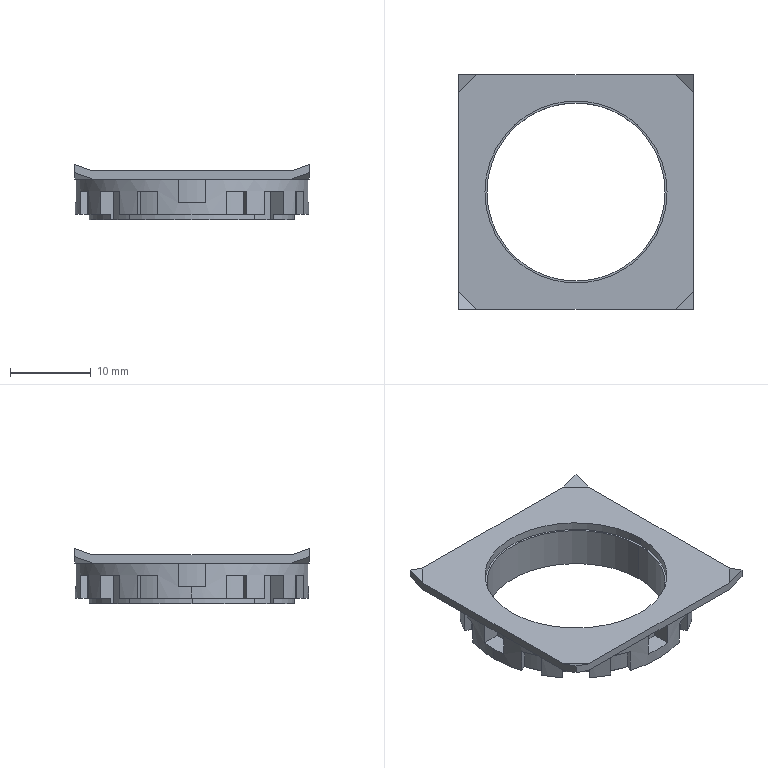Part | STEP file | A22NZ_2B[]_N[]A_NUT | 1 solid | 96 faces | box 29 x 29 x 6.8 mm | volume 1476 mm3 | plane 68 | cylinder 28 | commonest cylinder face diameters 27 x8 24.3 x5 25.4 x5 24.36 x4 22 x2 22.5 x2